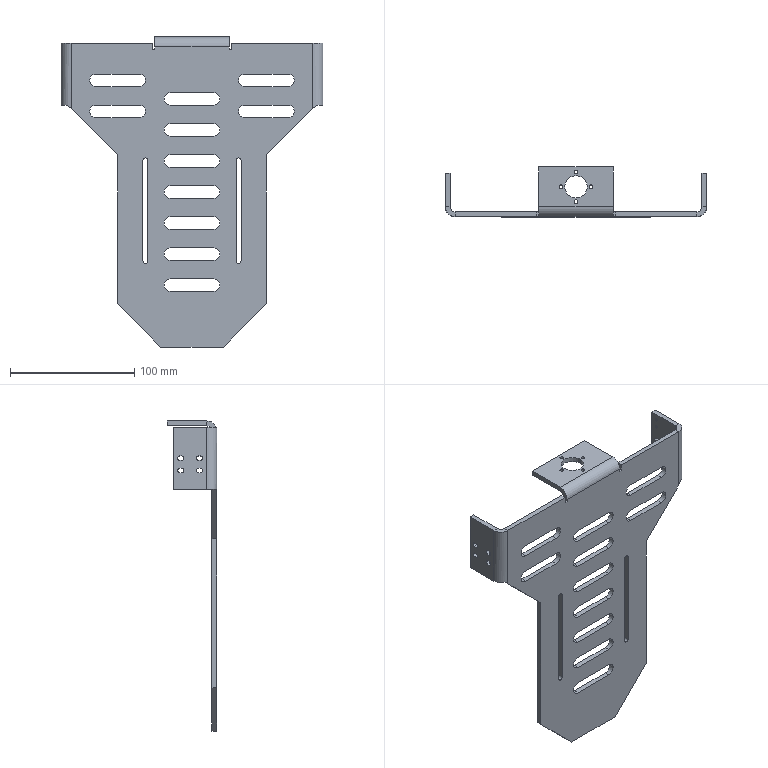Part | STEP file | Lift screen fixing plate V1.201001 | 1 solid | 152 faces | box 211 x 40 x 250 mm | volume 134618 mm3 | plane 80 | cylinder 72 | commonest cylinder face diameters 3.5 x24 10 x22 3 x8 4 x6 2.5 x4 8 x3